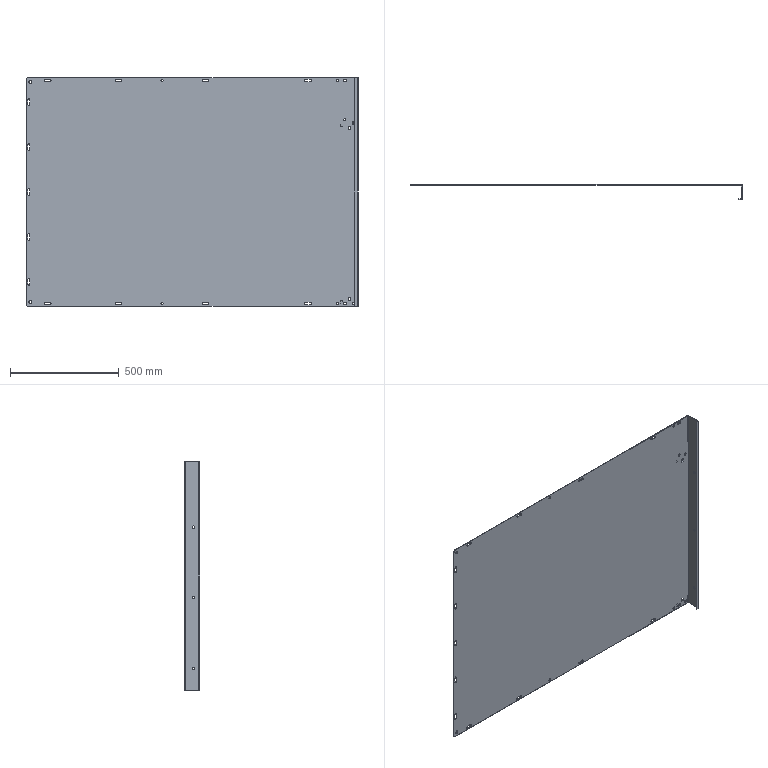Part | SolidWorks | features ICE 10, Cut 1, Fillet 1, FlatPattern 1, SMBaseFlange 1, SheetMetal 1 | 1 solid | 135 faces | box 1525 x 70 x 1050 mm | volume 5031582 mm3 | plane 70 | cylinder 65 | commonest cylinder face diameters 10 x41 10.5 x10 11 x4 12.8 x4 0.4 x2 6.4 x2